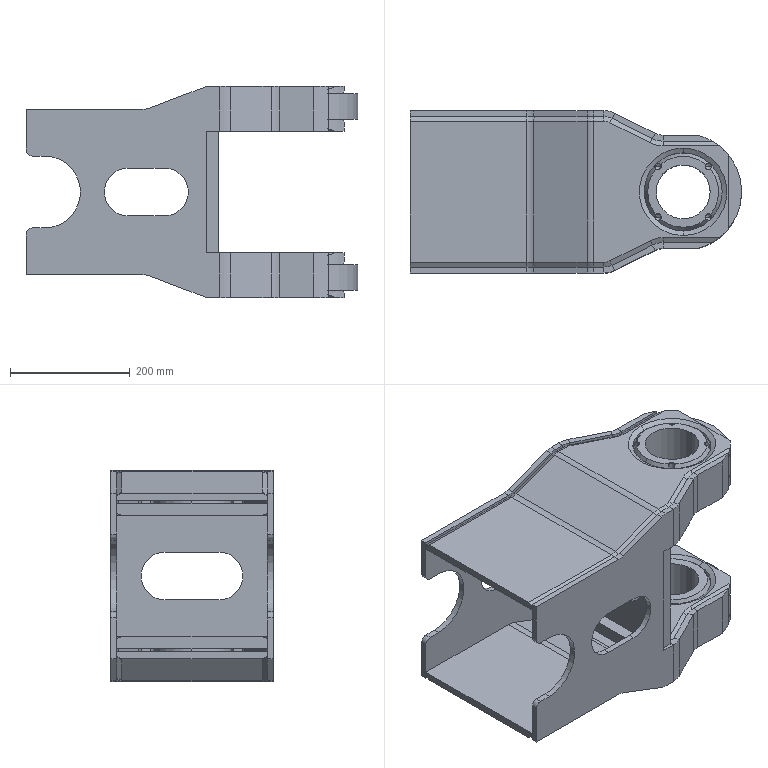Part | SolidWorks | features MirrorCompFeat 4, Cut 3, ReferencePattern 3, Chamfer 2, 3DProfileFeature 1, CirPattern 1, HoleWzd 1, MirrorPattern 1 | 11 solids | 414 faces | box 552.5 x 271 x 352 mm | volume 8203218 mm3 | plane 206 | cylinder 134 | cone 74 | commonest cylinder face diameters 10.2 x32 60 x28 80 x22 130 x18 195 x16 20 x4